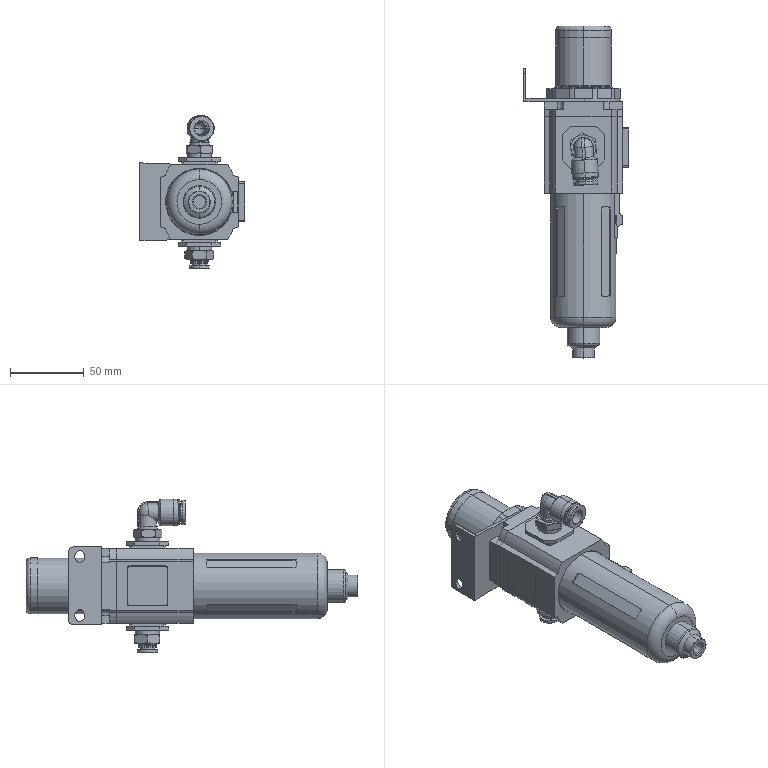Part | NX | features BREP 5 | 5 solids | 465 faces | box 72 x 225.5 x 104.5 mm | volume 282487 mm3 | plane 209 | cylinder 146 | cone 68 | torus 41 | sphere 1 | commonest cylinder face diameters 2 x26 40 x12 4 x11 8 x10 6.5 x6 50 x6